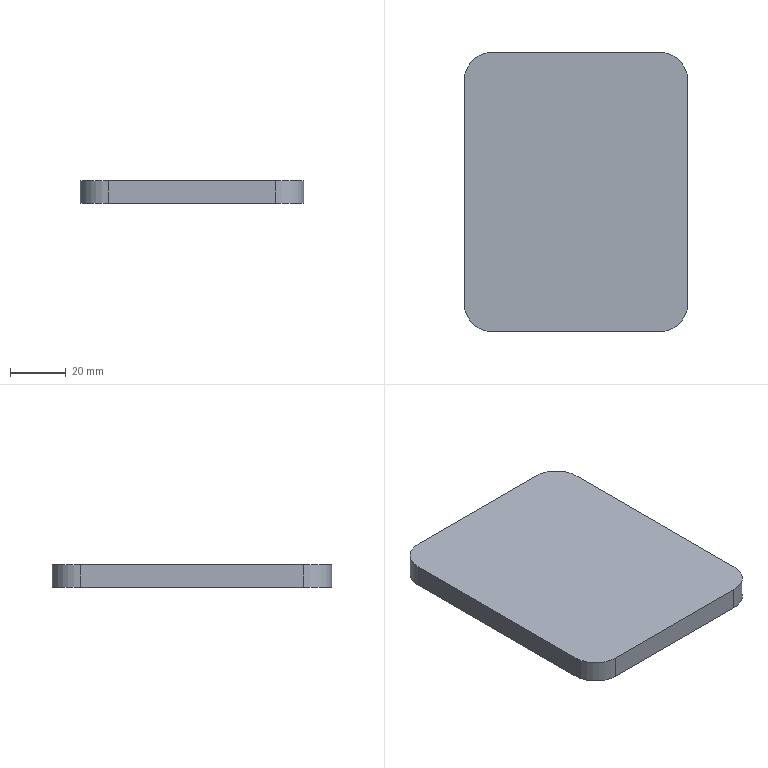Part | SolidWorks | features Extrusion 1 | 1 solid | 10 faces | box 80 x 100 x 8 mm | volume 63313 mm3 | plane 6 | cylinder 4 | commonest cylinder face diameters 20 x4
STEP:
#1=CARTESIAN_POINT('',(80.,90.,0.));
#2=VERTEX_POINT('',#1);
#3=CARTESIAN_POINT('',(70.,100.,0.));
#4=VERTEX_POINT('',#3);
#5=CARTESIAN_POINT('',(70.,90.,0.));
#6=DIRECTION('',(0.,0.,1.));
#7=DIRECTION('',(1.,0.,0.));
#8=AXIS2_PLACEMENT_3D('',#5,#6,#7);
#9=CIRCLE('',#8,10.);
#10=EDGE_CURVE('',#2,#4,#9,.T.);
#11=ORIENTED_EDGE('',*,*,#10,.T.);
#12=CARTESIAN_POINT('',(70.,100.,8.));
#13=VERTEX_POINT('',#12);
#14=CARTESIAN_POINT('',(70.,100.,8.));
#15=DIRECTION('',(0.,0.,-1.));
#16=VECTOR('',#15,1000.);
#17=LINE('',#14,#16);
#18=EDGE_CURVE('',#13,#4,#17,.T.);
#19=ORIENTED_EDGE('',*,*,#18,.F.);
#20=CARTESIAN_POINT('',(80.,90.,8.));
#21=VERTEX_POINT('',#20);
#22=CARTESIAN_POINT('',(70.,90.,8.));
#23=DIRECTION('',(0.,0.,1.));
#24=DIRECTION('',(1.,0.,0.));
#25=AXIS2_PLACEMENT_3D('',#22,#23,#24);
#26=CIRCLE('',#25,10.);
#27=EDGE_CURVE('',#21,#13,#26,.T.);
#28=ORIENTED_EDGE('',*,*,#27,.F.);
#29=CARTESIAN_POINT('',(80.,90.,8.));
#30=DIRECTION('',(0.,0.,-1.));
#31=VECTOR('',#30,1000.);
#32=LINE('',#29,#31);
#33=EDGE_CURVE('',#21,#2,#32,.T.);
#34=ORIENTED_EDGE('',*,*,#33,.T.);
#35=EDGE_LOOP('',(#11,#19,#28,#34));
#36=FACE_OUTER_BOUND('',#35,.T.);
#37=CARTESIAN_POINT('',(70.,90.,8.));
#38=DIRECTION('',(0.,0.,-1.));
#39=DIRECTION('',(-1.,0.,0.));
#40=AXIS2_PLACEMENT_3D('',#37,#38,#39);
#41=CYLINDRICAL_SURFACE('',#40,10.);
#42=ADVANCED_FACE('',(#36),#41,.T.);
#43=CARTESIAN_POINT('',(10.,100.,0.));
#44=VERTEX_POINT('',#43);
#45=CARTESIAN_POINT('',(10.,100.,0.));
#46=DIRECTION('',(-1.,0.,0.));
#47=VECTOR('',#46,1000.);
#48=LINE('',#45,#47);
#49=EDGE_CURVE('',#4,#44,#48,.T.);
#50=ORIENTED_EDGE('',*,*,#49,.T.);
#51=CARTESIAN_POINT('',(10.,100.,8.));
#52=VERTEX_POINT('',#51);
#53=CARTESIAN_POINT('',(10.,100.,8.));
#54=DIRECTION('',(0.,0.,-1.));
#55=VECTOR('',#54,1000.);
#56=LINE('',#53,#55);
#57=EDGE_CURVE('',#52,#44,#56,.T.);
#58=ORIENTED_EDGE('',*,*,#57,.F.);
#59=CARTESIAN_POINT('',(10.,100.,8.));
#60=DIRECTION('',(-1.,0.,0.));
#61=VECTOR('',#60,1000.);
#62=LINE('',#59,#61);
#63=EDGE_CURVE('',#13,#52,#62,.T.);
#64=ORIENTED_EDGE('',*,*,#63,.F.);
#65=ORIENTED_EDGE('',*,*,#18,.T.);
#66=EDGE_LOOP('',(#50,#58,#64,#65));
#67=FACE_OUTER_BOUND('',#66,.T.);
#68=CARTESIAN_POINT('',(10.,100.,8.));
#69=DIRECTION('',(0.,-1.,0.));
#70=DIRECTION('',(0.,0.,-1.));
#71=AXIS2_PLACEMENT_3D('',#68,#69,#70);
#72=PLANE('',#71);
#73=ADVANCED_FACE('',(#67),#72,.F.);
#74=CARTESIAN_POINT('',(0.,90.,0.));
#75=VERTEX_POINT('',#74);
#76=CARTESIAN_POINT('',(10.,90.,0.));
#77=DIRECTION('',(0.,0.,1.));
#78=DIRECTION('',(1.,0.,0.));
#79=AXIS2_PLACEMENT_3D('',#76,#77,#78);
#80=CIRCLE('',#79,10.);
#81=EDGE_CURVE('',#44,#75,#80,.T.);
#82=ORIENTED_EDGE('',*,*,#81,.T.);
#83=CARTESIAN_POINT('',(0.,90.,8.));
#84=VERTEX_POINT('',#83);
#85=CARTESIAN_POINT('',(0.,90.,8.));
#86=DIRECTION('',(0.,0.,-1.));
#87=VECTOR('',#86,1000.);
#88=LINE('',#85,#87);
#89=EDGE_CURVE('',#84,#75,#88,.T.);
#90=ORIENTED_EDGE('',*,*,#89,.F.);
#91=CARTESIAN_POINT('',(10.,90.,8.));
#92=DIRECTION('',(0.,0.,1.));
#93=DIRECTION('',(1.,0.,0.));
#94=AXIS2_PLACEMENT_3D('',#91,#92,#93);
#95=CIRCLE('',#94,10.);
#96=EDGE_CURVE('',#52,#84,#95,.T.);
#97=ORIENTED_EDGE('',*,*,#96,.F.);
#98=ORIENTED_EDGE('',*,*,#57,.T.);
#99=EDGE_LOOP('',(#82,#90,#97,#98));
#100=FACE_OUTER_BOUND('',#99,.T.);
#101=CARTESIAN_POINT('',(10.,90.,8.));
#102=DIRECTION('',(0.,0.,-1.));
#103=DIRECTION('',(-1.,0.,0.));
#104=AXIS2_PLACEMENT_3D('',#101,#102,#103);
#105=CYLINDRICAL_SURFACE('',#104,10.);
#106=ADVANCED_FACE('',(#100),#105,.T.);
#107=CARTESIAN_POINT('',(0.,10.,0.));
#108=VERTEX_POINT('',#107);
#109=CARTESIAN_POINT('',(0.,10.,0.));
#110=DIRECTION('',(0.,-1.,0.));
#111=VECTOR('',#110,1000.);
#112=LINE('',#109,#111);
#113=EDGE_CURVE('',#75,#108,#112,.T.);
#114=ORIENTED_EDGE('',*,*,#113,.T.);
#115=CARTESIAN_POINT('',(0.,10.,8.));
#116=VERTEX_POINT('',#115);
#117=CARTESIAN_POINT('',(0.,10.,8.));
#118=DIRECTION('',(0.,0.,-1.));
#119=VECTOR('',#118,1000.);
#120=LINE('',#117,#119);
#121=EDGE_CURVE('',#116,#108,#120,.T.);
#122=ORIENTED_EDGE('',*,*,#121,.F.);
#123=CARTESIAN_POINT('',(0.,10.,8.));
#124=DIRECTION('',(0.,-1.,0.));
#125=VECTOR('',#124,1000.);
#126=LINE('',#123,#125);
#127=EDGE_CURVE('',#84,#116,#126,.T.);
#128=ORIENTED_EDGE('',*,*,#127,.F.);
#129=ORIENTED_EDGE('',*,*,#89,.T.);
#130=EDGE_LOOP('',(#114,#122,#128,#129));
#131=FACE_OUTER_BOUND('',#130,.T.);
#132=CARTESIAN_POINT('',(0.,10.,8.));
#133=DIRECTION('',(1.,0.,0.));
#134=DIRECTION('',(0.,0.,-1.));
#135=AXIS2_PLACEMENT_3D('',#132,#133,#134);
#136=PLANE('',#135);
#137=ADVANCED_FACE('',(#131),#136,.F.);
#138=CARTESIAN_POINT('',(10.,0.,0.));
#139=VERTEX_POINT('',#138);
#140=CARTESIAN_POINT('',(10.,10.,0.));
#141=DIRECTION('',(0.,0.,1.));
#142=DIRECTION('',(-1.,0.,0.));
#143=AXIS2_PLACEMENT_3D('',#140,#141,#142);
#144=CIRCLE('',#143,10.);
#145=EDGE_CURVE('',#108,#139,#144,.T.);
#146=ORIENTED_EDGE('',*,*,#145,.T.);
#147=CARTESIAN_POINT('',(10.,0.,8.));
#148=VERTEX_POINT('',#147);
#149=CARTESIAN_POINT('',(10.,0.,8.));
#150=DIRECTION('',(0.,0.,-1.));
#151=VECTOR('',#150,1000.);
#152=LINE('',#149,#151);
#153=EDGE_CURVE('',#148,#139,#152,.T.);
#154=ORIENTED_EDGE('',*,*,#153,.F.);
#155=CARTESIAN_POINT('',(10.,10.,8.));
#156=DIRECTION('',(0.,0.,1.));
#157=DIRECTION('',(-1.,0.,0.));
#158=AXIS2_PLACEMENT_3D('',#155,#156,#157);
#159=CIRCLE('',#158,10.);
#160=EDGE_CURVE('',#116,#148,#159,.T.);
#161=ORIENTED_EDGE('',*,*,#160,.F.);
#162=ORIENTED_EDGE('',*,*,#121,.T.);
#163=EDGE_LOOP('',(#146,#154,#161,#162));
#164=FACE_OUTER_BOUND('',#163,.T.);
#165=CARTESIAN_POINT('',(10.,10.,8.));
#166=DIRECTION('',(0.,0.,-1.));
#167=DIRECTION('',(-1.,0.,0.));
#168=AXIS2_PLACEMENT_3D('',#165,#166,#167);
#169=CYLINDRICAL_SURFACE('',#168,10.);
#170=ADVANCED_FACE('',(#164),#169,.T.);
#171=CARTESIAN_POINT('',(70.,0.,0.));
#172=VERTEX_POINT('',#171);
#173=CARTESIAN_POINT('',(10.,0.,0.));
#174=DIRECTION('',(1.,0.,0.));
#175=VECTOR('',#174,1000.);
#176=LINE('',#173,#175);
#177=EDGE_CURVE('',#139,#172,#176,.T.);
#178=ORIENTED_EDGE('',*,*,#177,.T.);
#179=CARTESIAN_POINT('',(70.,0.,8.));
#180=VERTEX_POINT('',#179);
#181=CARTESIAN_POINT('',(70.,0.,8.));
#182=DIRECTION('',(0.,0.,-1.));
#183=VECTOR('',#182,1000.);
#184=LINE('',#181,#183);
#185=EDGE_CURVE('',#180,#172,#184,.T.);
#186=ORIENTED_EDGE('',*,*,#185,.F.);
#187=CARTESIAN_POINT('',(10.,0.,8.));
#188=DIRECTION('',(1.,0.,0.));
#189=VECTOR('',#188,1000.);
#190=LINE('',#187,#189);
#191=EDGE_CURVE('',#148,#180,#190,.T.);
#192=ORIENTED_EDGE('',*,*,#191,.F.);
#193=ORIENTED_EDGE('',*,*,#153,.T.);
#194=EDGE_LOOP('',(#178,#186,#192,#193));
#195=FACE_OUTER_BOUND('',#194,.T.);
#196=CARTESIAN_POINT('',(10.,0.,8.));
#197=DIRECTION('',(0.,1.,0.));
#198=DIRECTION('',(0.,0.,1.));
#199=AXIS2_PLACEMENT_3D('',#196,#197,#198);
#200=PLANE('',#199);
#201=ADVANCED_FACE('',(#195),#200,.F.);
#202=CARTESIAN_POINT('',(80.,10.,0.));
#203=VERTEX_POINT('',#202);
#204=CARTESIAN_POINT('',(70.,10.,0.));
#205=DIRECTION('',(0.,0.,1.));
#206=DIRECTION('',(-1.,0.,0.));
#207=AXIS2_PLACEMENT_3D('',#204,#205,#206);
#208=CIRCLE('',#207,10.);
#209=EDGE_CURVE('',#172,#203,#208,.T.);
#210=ORIENTED_EDGE('',*,*,#209,.T.);
#211=CARTESIAN_POINT('',(80.,10.,8.));
#212=VERTEX_POINT('',#211);
#213=CARTESIAN_POINT('',(80.,10.,8.));
#214=DIRECTION('',(0.,0.,-1.));
#215=VECTOR('',#214,1000.);
#216=LINE('',#213,#215);
#217=EDGE_CURVE('',#212,#203,#216,.T.);
#218=ORIENTED_EDGE('',*,*,#217,.F.);
#219=CARTESIAN_POINT('',(70.,10.,8.));
#220=DIRECTION('',(0.,0.,1.));
#221=DIRECTION('',(-1.,0.,0.));
#222=AXIS2_PLACEMENT_3D('',#219,#220,#221);
#223=CIRCLE('',#222,10.);
#224=EDGE_CURVE('',#180,#212,#223,.T.);
#225=ORIENTED_EDGE('',*,*,#224,.F.);
#226=ORIENTED_EDGE('',*,*,#185,.T.);
#227=EDGE_LOOP('',(#210,#218,#225,#226));
#228=FACE_OUTER_BOUND('',#227,.T.);
#229=CARTESIAN_POINT('',(70.,10.,8.));
#230=DIRECTION('',(0.,0.,-1.));
#231=DIRECTION('',(-1.,0.,0.));
#232=AXIS2_PLACEMENT_3D('',#229,#230,#231);
#233=CYLINDRICAL_SURFACE('',#232,10.);
#234=ADVANCED_FACE('',(#228),#233,.T.);
#235=CARTESIAN_POINT('',(80.,10.,0.));
#236=DIRECTION('',(0.,1.,0.));
#237=VECTOR('',#236,1000.);
#238=LINE('',#235,#237);
#239=EDGE_CURVE('',#203,#2,#238,.T.);
#240=ORIENTED_EDGE('',*,*,#239,.T.);
#241=ORIENTED_EDGE('',*,*,#33,.F.);
#242=CARTESIAN_POINT('',(80.,10.,8.));
#243=DIRECTION('',(0.,1.,0.));
#244=VECTOR('',#243,1000.);
#245=LINE('',#242,#244);
#246=EDGE_CURVE('',#212,#21,#245,.T.);
#247=ORIENTED_EDGE('',*,*,#246,.F.);
#248=ORIENTED_EDGE('',*,*,#217,.T.);
#249=EDGE_LOOP('',(#240,#241,#247,#248));
#250=FACE_OUTER_BOUND('',#249,.T.);
#251=CARTESIAN_POINT('',(80.,10.,8.));
#252=DIRECTION('',(-1.,0.,0.));
#253=DIRECTION('',(0.,-1.,0.));
#254=AXIS2_PLACEMENT_3D('',#251,#252,#253);
#255=PLANE('',#254);
#256=ADVANCED_FACE('',(#250),#255,.F.);
#257=ORIENTED_EDGE('',*,*,#27,.T.);
#258=ORIENTED_EDGE('',*,*,#63,.T.);
#259=ORIENTED_EDGE('',*,*,#96,.T.);
#260=ORIENTED_EDGE('',*,*,#127,.T.);
#261=ORIENTED_EDGE('',*,*,#160,.T.);
#262=ORIENTED_EDGE('',*,*,#191,.T.);
#263=ORIENTED_EDGE('',*,*,#224,.T.);
#264=ORIENTED_EDGE('',*,*,#246,.T.);
#265=EDGE_LOOP('',(#257,#258,#259,#260,#261,#262,#263,#264));
#266=FACE_OUTER_BOUND('',#265,.T.);
#267=CARTESIAN_POINT('',(70.,90.,8.));
#268=DIRECTION('',(0.,0.,1.));
#269=DIRECTION('',(1.,0.,0.));
#270=AXIS2_PLACEMENT_3D('',#267,#268,#269);
#271=PLANE('',#270);
#272=ADVANCED_FACE('',(#266),#271,.T.);
#273=ORIENTED_EDGE('',*,*,#10,.F.);
#274=ORIENTED_EDGE('',*,*,#239,.F.);
#275=ORIENTED_EDGE('',*,*,#209,.F.);
#276=ORIENTED_EDGE('',*,*,#177,.F.);
#277=ORIENTED_EDGE('',*,*,#145,.F.);
#278=ORIENTED_EDGE('',*,*,#113,.F.);
#279=ORIENTED_EDGE('',*,*,#81,.F.);
#280=ORIENTED_EDGE('',*,*,#49,.F.);
#281=EDGE_LOOP('',(#273,#274,#275,#276,#277,#278,#279,#280));
#282=FACE_OUTER_BOUND('',#281,.T.);
#283=CARTESIAN_POINT('',(70.,90.,0.));
#284=DIRECTION('',(0.,0.,1.));
#285=DIRECTION('',(1.,0.,0.));
#286=AXIS2_PLACEMENT_3D('',#283,#284,#285);
#287=PLANE('',#286);
#288=ADVANCED_FACE('',(#282),#287,.F.);
#289=CLOSED_SHELL('',(#42,#73,#106,#137,#170,#201,#234,#256,#272,#288));
#290=MANIFOLD_SOLID_BREP('',#289);
#291=CARTESIAN_POINT('',(0.,0.,0.));
#292=DIRECTION('',(0.,0.,1.));
#293=DIRECTION('',(1.,0.,0.));
#294=AXIS2_PLACEMENT_3D('',#291,#292,#293);
#295=(LENGTH_UNIT()NAMED_UNIT(*)SI_UNIT(.MILLI.,.METRE.));
#296=UNCERTAINTY_MEASURE_WITH_UNIT(LENGTH_MEASURE(0.00001),#295,'','');
#297=(NAMED_UNIT(*)PLANE_ANGLE_UNIT()SI_UNIT($,.RADIAN.));
#298=(NAMED_UNIT(*)SI_UNIT($,.STERADIAN.)SOLID_ANGLE_UNIT());
#299=(GEOMETRIC_REPRESENTATION_CONTEXT(3)GLOBAL_UNCERTAINTY_ASSIGNED_CONTEXT((#296))GLOBAL_UNIT_ASSIGNED_CONTEXT((#295,#297,#298))REPRESENTATION_CONTEXT('',''));
#300=ADVANCED_BREP_SHAPE_REPRESENTATION('',(#290,#294),#299);